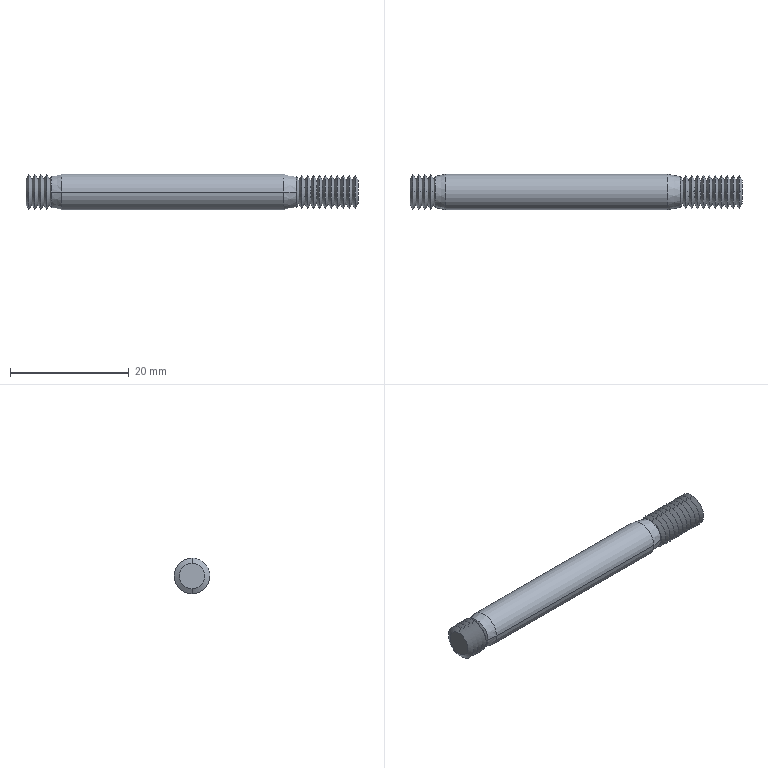Part | SolidWorks | features LPattern 2, RevCut 2, Chamfer 1, Revolution 1 | 1 solid | 80 faces | box 56 x 6 x 6 mm | volume 1438 mm3 | cone 68 | cylinder 10 | plane 2 | commonest cylinder face diameters 6 x10